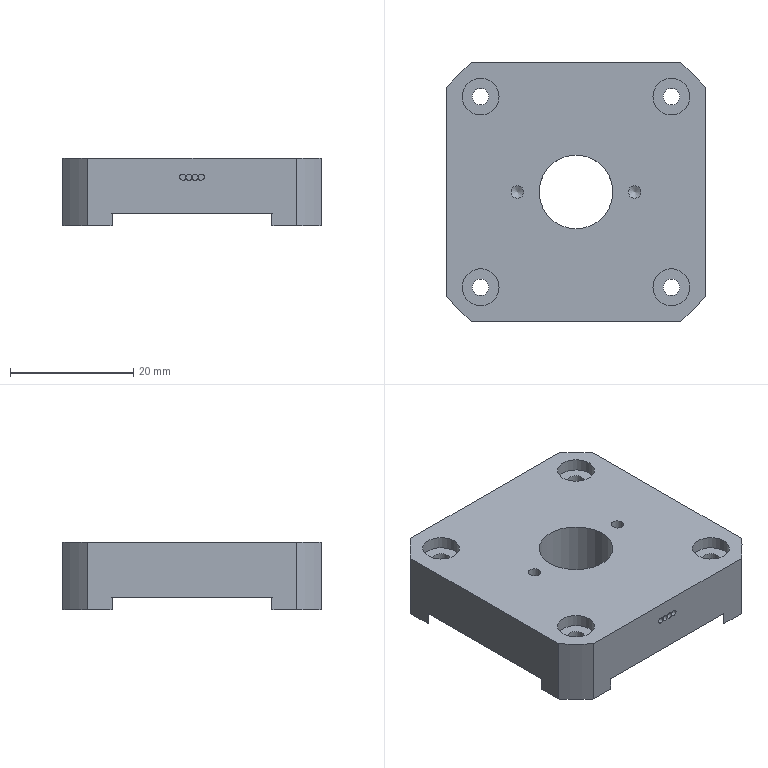Part | NX | 1 solid | 43 faces | box 42 x 42 x 11 mm | volume 14366 mm3 | plane 22 | cylinder 19 | cone 2 | commonest cylinder face diameters 1 x4 2.7 x4 6 x4 54 x4 2.013 x2 12 x1
STEP:
#1=CARTESIAN_POINT('',(-1.,-21.,7.9));
#2=VERTEX_POINT('',#1);
#3=CARTESIAN_POINT('',(-1.5,-21.,7.9));
#4=DIRECTION('',(0.,-1.,0.));
#5=DIRECTION('',(0.,0.,-1.));
#6=AXIS2_PLACEMENT_3D('',#3,#4,#5);
#7=CIRCLE('',#6,0.5);
#8=EDGE_CURVE('',#2,#2,#7,.T.);
#9=ORIENTED_EDGE('',*,*,#8,.T.);
#10=EDGE_LOOP('',(#9));
#11=FACE_BOUND('',#10,.T.);
#12=CARTESIAN_POINT('',(-1.5,-18.,7.4));
#13=VERTEX_POINT('',#12);
#14=CARTESIAN_POINT('',(-1.5,-18.,7.9));
#15=DIRECTION('',(0.,-1.,0.));
#16=DIRECTION('',(0.,0.,-1.));
#17=AXIS2_PLACEMENT_3D('',#14,#15,#16);
#18=CIRCLE('',#17,0.5);
#19=EDGE_CURVE('',#13,#13,#18,.T.);
#20=ORIENTED_EDGE('',*,*,#19,.F.);
#21=EDGE_LOOP('',(#20));
#22=FACE_BOUND('',#21,.T.);
#23=CARTESIAN_POINT('',(-1.5,-19.5,7.9));
#24=DIRECTION('',(0.,-1.,0.));
#25=DIRECTION('',(0.,0.,-1.));
#26=AXIS2_PLACEMENT_3D('',#23,#24,#25);
#27=CYLINDRICAL_SURFACE('',#26,0.5);
#28=ADVANCED_FACE('',(#11,#22),#27,.F.);
#29=ORIENTED_EDGE('',*,*,#19,.T.);
#30=EDGE_LOOP('',(#29));
#31=FACE_BOUND('',#30,.T.);
#32=CARTESIAN_POINT('',(-1.5,-18.,8.4));
#33=DIRECTION('',(0.,1.,0.));
#34=DIRECTION('',(0.,0.,1.));
#35=AXIS2_PLACEMENT_3D('',#32,#33,#34);
#36=PLANE('',#35);
#37=ADVANCED_FACE('',(#31),#36,.F.);
#38=CARTESIAN_POINT('',(-0.5,-18.,7.4));
#39=VERTEX_POINT('',#38);
#40=CARTESIAN_POINT('',(-0.5,-18.,7.9));
#41=DIRECTION('',(0.,-1.,0.));
#42=DIRECTION('',(0.,0.,-1.));
#43=AXIS2_PLACEMENT_3D('',#40,#41,#42);
#44=CIRCLE('',#43,0.5);
#45=EDGE_CURVE('',#39,#39,#44,.T.);
#46=ORIENTED_EDGE('',*,*,#45,.T.);
#47=EDGE_LOOP('',(#46));
#48=FACE_BOUND('',#47,.T.);
#49=CARTESIAN_POINT('',(-0.5,-18.,8.4));
#50=DIRECTION('',(0.,1.,0.));
#51=DIRECTION('',(0.,0.,1.));
#52=AXIS2_PLACEMENT_3D('',#49,#50,#51);
#53=PLANE('',#52);
#54=ADVANCED_FACE('',(#48),#53,.F.);
#55=CARTESIAN_POINT('',(1.5,-18.,7.4));
#56=VERTEX_POINT('',#55);
#57=CARTESIAN_POINT('',(1.5,-18.,7.9));
#58=DIRECTION('',(0.,-1.,0.));
#59=DIRECTION('',(0.,0.,-1.));
#60=AXIS2_PLACEMENT_3D('',#57,#58,#59);
#61=CIRCLE('',#60,0.5);
#62=EDGE_CURVE('',#56,#56,#61,.T.);
#63=ORIENTED_EDGE('',*,*,#62,.T.);
#64=EDGE_LOOP('',(#63));
#65=FACE_BOUND('',#64,.T.);
#66=CARTESIAN_POINT('',(1.5,-18.,8.4));
#67=DIRECTION('',(0.,1.,0.));
#68=DIRECTION('',(0.,0.,1.));
#69=AXIS2_PLACEMENT_3D('',#66,#67,#68);
#70=PLANE('',#69);
#71=ADVANCED_FACE('',(#65),#70,.F.);
#72=CARTESIAN_POINT('',(-9.525,0.,7.395));
#73=VERTEX_POINT('',#72);
#74=VERTEX_LOOP('',#73);
#75=FACE_BOUND('',#74,.T.);
#76=CARTESIAN_POINT('',(-8.518,0.,8.));
#77=VERTEX_POINT('',#76);
#78=CARTESIAN_POINT('',(-9.525,0.,8.));
#79=DIRECTION('',(0.,0.,1.));
#80=DIRECTION('',(1.,0.,0.));
#81=AXIS2_PLACEMENT_3D('',#78,#79,#80);
#82=CIRCLE('',#81,1.006);
#83=EDGE_CURVE('',#77,#77,#82,.T.);
#84=ORIENTED_EDGE('',*,*,#83,.T.);
#85=EDGE_LOOP('',(#84));
#86=FACE_BOUND('',#85,.T.);
#87=CARTESIAN_POINT('',(-9.525,0.,8.));
#88=DIRECTION('',(0.,0.,1.));
#89=DIRECTION('',(1.,0.,0.));
#90=AXIS2_PLACEMENT_3D('',#87,#88,#89);
#91=CONICAL_SURFACE('',#90,1.007,1.03);
#92=ADVANCED_FACE('',(#75,#86),#91,.F.);
#93=CARTESIAN_POINT('',(9.525,0.,7.395));
#94=VERTEX_POINT('',#93);
#95=VERTEX_LOOP('',#94);
#96=FACE_BOUND('',#95,.T.);
#97=CARTESIAN_POINT('',(10.531,0.,8.));
#98=VERTEX_POINT('',#97);
#99=CARTESIAN_POINT('',(9.525,0.,8.));
#100=DIRECTION('',(0.,0.,1.));
#101=DIRECTION('',(1.,0.,0.));
#102=AXIS2_PLACEMENT_3D('',#99,#100,#101);
#103=CIRCLE('',#102,1.006);
#104=EDGE_CURVE('',#98,#98,#103,.T.);
#105=ORIENTED_EDGE('',*,*,#104,.T.);
#106=EDGE_LOOP('',(#105));
#107=FACE_BOUND('',#106,.T.);
#108=CARTESIAN_POINT('',(9.525,0.,8.));
#109=DIRECTION('',(0.,0.,1.));
#110=DIRECTION('',(1.,0.,0.));
#111=AXIS2_PLACEMENT_3D('',#108,#109,#110);
#112=CONICAL_SURFACE('',#111,1.006,1.03);
#113=ADVANCED_FACE('',(#96,#107),#112,.F.);
#114=CARTESIAN_POINT('',(-14.15,15.5,9.));
#115=VERTEX_POINT('',#114);
#116=CARTESIAN_POINT('',(-15.5,15.5,9.));
#117=DIRECTION('',(0.,0.,1.));
#118=DIRECTION('',(1.,0.,0.));
#119=AXIS2_PLACEMENT_3D('',#116,#117,#118);
#120=CIRCLE('',#119,1.35);
#121=EDGE_CURVE('',#115,#115,#120,.T.);
#122=ORIENTED_EDGE('',*,*,#121,.F.);
#123=EDGE_LOOP('',(#122));
#124=FACE_BOUND('',#123,.T.);
#125=CARTESIAN_POINT('',(-12.5,15.5,9.));
#126=VERTEX_POINT('',#125);
#127=CARTESIAN_POINT('',(-15.5,15.5,9.));
#128=DIRECTION('',(0.,0.,1.));
#129=DIRECTION('',(1.,0.,0.));
#130=AXIS2_PLACEMENT_3D('',#127,#128,#129);
#131=CIRCLE('',#130,3.);
#132=EDGE_CURVE('',#126,#126,#131,.T.);
#133=ORIENTED_EDGE('',*,*,#132,.T.);
#134=EDGE_LOOP('',(#133));
#135=FACE_BOUND('',#134,.T.);
#136=CARTESIAN_POINT('',(-15.5,18.5,9.));
#137=DIRECTION('',(0.,0.,-1.));
#138=DIRECTION('',(-1.,0.,0.));
#139=AXIS2_PLACEMENT_3D('',#136,#137,#138);
#140=PLANE('',#139);
#141=ADVANCED_FACE('',(#124,#135),#140,.F.);
#142=CARTESIAN_POINT('',(16.85,15.5,9.));
#143=VERTEX_POINT('',#142);
#144=CARTESIAN_POINT('',(15.5,15.5,9.));
#145=DIRECTION('',(0.,0.,1.));
#146=DIRECTION('',(1.,0.,0.));
#147=AXIS2_PLACEMENT_3D('',#144,#145,#146);
#148=CIRCLE('',#147,1.35);
#149=EDGE_CURVE('',#143,#143,#148,.T.);
#150=ORIENTED_EDGE('',*,*,#149,.F.);
#151=EDGE_LOOP('',(#150));
#152=FACE_BOUND('',#151,.T.);
#153=CARTESIAN_POINT('',(18.5,15.5,9.));
#154=VERTEX_POINT('',#153);
#155=CARTESIAN_POINT('',(15.5,15.5,9.));
#156=DIRECTION('',(0.,0.,1.));
#157=DIRECTION('',(1.,0.,0.));
#158=AXIS2_PLACEMENT_3D('',#155,#156,#157);
#159=CIRCLE('',#158,3.);
#160=EDGE_CURVE('',#154,#154,#159,.T.);
#161=ORIENTED_EDGE('',*,*,#160,.T.);
#162=EDGE_LOOP('',(#161));
#163=FACE_BOUND('',#162,.T.);
#164=CARTESIAN_POINT('',(15.5,18.5,9.));
#165=DIRECTION('',(0.,0.,-1.));
#166=DIRECTION('',(-1.,0.,0.));
#167=AXIS2_PLACEMENT_3D('',#164,#165,#166);
#168=PLANE('',#167);
#169=ADVANCED_FACE('',(#152,#163),#168,.F.);
#170=CARTESIAN_POINT('',(-14.15,-15.5,9.));
#171=VERTEX_POINT('',#170);
#172=CARTESIAN_POINT('',(-15.5,-15.5,9.));
#173=DIRECTION('',(0.,0.,1.));
#174=DIRECTION('',(1.,0.,0.));
#175=AXIS2_PLACEMENT_3D('',#172,#173,#174);
#176=CIRCLE('',#175,1.35);
#177=EDGE_CURVE('',#171,#171,#176,.T.);
#178=ORIENTED_EDGE('',*,*,#177,.F.);
#179=EDGE_LOOP('',(#178));
#180=FACE_BOUND('',#179,.T.);
#181=CARTESIAN_POINT('',(-12.5,-15.5,9.));
#182=VERTEX_POINT('',#181);
#183=CARTESIAN_POINT('',(-15.5,-15.5,9.));
#184=DIRECTION('',(0.,0.,1.));
#185=DIRECTION('',(1.,0.,0.));
#186=AXIS2_PLACEMENT_3D('',#183,#184,#185);
#187=CIRCLE('',#186,3.);
#188=EDGE_CURVE('',#182,#182,#187,.T.);
#189=ORIENTED_EDGE('',*,*,#188,.T.);
#190=EDGE_LOOP('',(#189));
#191=FACE_BOUND('',#190,.T.);
#192=CARTESIAN_POINT('',(-15.5,-12.5,9.));
#193=DIRECTION('',(0.,0.,-1.));
#194=DIRECTION('',(-1.,0.,0.));
#195=AXIS2_PLACEMENT_3D('',#192,#193,#194);
#196=PLANE('',#195);
#197=ADVANCED_FACE('',(#180,#191),#196,.F.);
#198=CARTESIAN_POINT('',(16.85,-15.5,9.));
#199=VERTEX_POINT('',#198);
#200=CARTESIAN_POINT('',(15.5,-15.5,9.));
#201=DIRECTION('',(0.,0.,1.));
#202=DIRECTION('',(1.,0.,0.));
#203=AXIS2_PLACEMENT_3D('',#200,#201,#202);
#204=CIRCLE('',#203,1.35);
#205=EDGE_CURVE('',#199,#199,#204,.T.);
#206=ORIENTED_EDGE('',*,*,#205,.F.);
#207=EDGE_LOOP('',(#206));
#208=FACE_BOUND('',#207,.T.);
#209=CARTESIAN_POINT('',(18.5,-15.5,9.));
#210=VERTEX_POINT('',#209);
#211=CARTESIAN_POINT('',(15.5,-15.5,9.));
#212=DIRECTION('',(0.,0.,1.));
#213=DIRECTION('',(1.,0.,0.));
#214=AXIS2_PLACEMENT_3D('',#211,#212,#213);
#215=CIRCLE('',#214,3.);
#216=EDGE_CURVE('',#210,#210,#215,.T.);
#217=ORIENTED_EDGE('',*,*,#216,.T.);
#218=EDGE_LOOP('',(#217));
#219=FACE_BOUND('',#218,.T.);
#220=CARTESIAN_POINT('',(15.5,-12.5,9.));
#221=DIRECTION('',(0.,0.,-1.));
#222=DIRECTION('',(-1.,0.,0.));
#223=AXIS2_PLACEMENT_3D('',#220,#221,#222);
#224=PLANE('',#223);
#225=ADVANCED_FACE('',(#208,#219),#224,.F.);
#226=CARTESIAN_POINT('',(16.971,21.,0.));
#227=VERTEX_POINT('',#226);
#228=CARTESIAN_POINT('',(13.,21.,0.));
#229=VERTEX_POINT('',#228);
#230=CARTESIAN_POINT('',(-16.971,21.,0.));
#231=DIRECTION('',(1.,0.,0.));
#232=VECTOR('',#231,1000.);
#233=LINE('',#230,#232);
#234=EDGE_CURVE('',#227,#229,#233,.F.);
#235=ORIENTED_EDGE('',*,*,#234,.F.);
#236=CARTESIAN_POINT('',(21.,16.971,0.));
#237=VERTEX_POINT('',#236);
#238=CARTESIAN_POINT('',(0.,0.,0.));
#239=DIRECTION('',(0.,0.,1.));
#240=DIRECTION('',(1.,0.,0.));
#241=AXIS2_PLACEMENT_3D('',#238,#239,#240);
#242=CIRCLE('',#241,27.);
#243=EDGE_CURVE('',#237,#227,#242,.T.);
#244=ORIENTED_EDGE('',*,*,#243,.F.);
#245=CARTESIAN_POINT('',(21.,13.,0.));
#246=VERTEX_POINT('',#245);
#247=CARTESIAN_POINT('',(21.,16.971,0.));
#248=DIRECTION('',(0.,1.,0.));
#249=VECTOR('',#248,1000.);
#250=LINE('',#247,#249);
#251=EDGE_CURVE('',#246,#237,#250,.T.);
#252=ORIENTED_EDGE('',*,*,#251,.F.);
#253=CARTESIAN_POINT('',(13.,21.,0.));
#254=DIRECTION('',(0.7071,-0.7071,0.));
#255=VECTOR('',#254,1000.);
#256=LINE('',#253,#255);
#257=EDGE_CURVE('',#229,#246,#256,.T.);
#258=ORIENTED_EDGE('',*,*,#257,.F.);
#259=EDGE_LOOP('',(#235,#244,#252,#258));
#260=FACE_BOUND('',#259,.T.);
#261=CARTESIAN_POINT('',(0.,0.,0.));
#262=DIRECTION('',(0.,0.,1.));
#263=DIRECTION('',(1.,0.,0.));
#264=AXIS2_PLACEMENT_3D('',#261,#262,#263);
#265=PLANE('',#264);
#266=ADVANCED_FACE('',(#260),#265,.F.);
#267=CARTESIAN_POINT('',(-21.,16.971,0.));
#268=VERTEX_POINT('',#267);
#269=CARTESIAN_POINT('',(-21.,13.,0.));
#270=VERTEX_POINT('',#269);
#271=CARTESIAN_POINT('',(-21.,-16.971,0.));
#272=DIRECTION('',(0.,1.,0.));
#273=VECTOR('',#272,1000.);
#274=LINE('',#271,#273);
#275=EDGE_CURVE('',#268,#270,#274,.F.);
#276=ORIENTED_EDGE('',*,*,#275,.F.);
#277=CARTESIAN_POINT('',(-16.971,21.,0.));
#278=VERTEX_POINT('',#277);
#279=CARTESIAN_POINT('',(0.,0.,0.));
#280=DIRECTION('',(0.,0.,1.));
#281=DIRECTION('',(1.,0.,0.));
#282=AXIS2_PLACEMENT_3D('',#279,#280,#281);
#283=CIRCLE('',#282,27.);
#284=EDGE_CURVE('',#278,#268,#283,.T.);
#285=ORIENTED_EDGE('',*,*,#284,.F.);
#286=CARTESIAN_POINT('',(-13.,21.,0.));
#287=VERTEX_POINT('',#286);
#288=CARTESIAN_POINT('',(-16.971,21.,0.));
#289=DIRECTION('',(1.,0.,0.));
#290=VECTOR('',#289,1000.);
#291=LINE('',#288,#290);
#292=EDGE_CURVE('',#287,#278,#291,.F.);
#293=ORIENTED_EDGE('',*,*,#292,.F.);
#294=CARTESIAN_POINT('',(-21.,13.,0.));
#295=DIRECTION('',(-0.7071,-0.7071,0.));
#296=VECTOR('',#295,1000.);
#297=LINE('',#294,#296);
#298=EDGE_CURVE('',#287,#270,#297,.T.);
#299=ORIENTED_EDGE('',*,*,#298,.T.);
#300=EDGE_LOOP('',(#276,#285,#293,#299));
#301=FACE_BOUND('',#300,.T.);
#302=CARTESIAN_POINT('',(0.,0.,0.));
#303=DIRECTION('',(0.,0.,1.));
#304=DIRECTION('',(1.,0.,0.));
#305=AXIS2_PLACEMENT_3D('',#302,#303,#304);
#306=PLANE('',#305);
#307=ADVANCED_FACE('',(#301),#306,.F.);
#308=ORIENTED_EDGE('',*,*,#284,.T.);
#309=CARTESIAN_POINT('',(-21.,16.971,11.));
#310=VERTEX_POINT('',#309);
#311=CARTESIAN_POINT('',(-21.,16.971,0.));
#312=DIRECTION('',(0.,0.,1.));
#313=VECTOR('',#312,1000.);
#314=LINE('',#311,#313);
#315=EDGE_CURVE('',#310,#268,#314,.F.);
#316=ORIENTED_EDGE('',*,*,#315,.F.);
#317=CARTESIAN_POINT('',(-16.971,21.,11.));
#318=VERTEX_POINT('',#317);
#319=CARTESIAN_POINT('',(0.,0.,11.));
#320=DIRECTION('',(0.,0.,1.));
#321=DIRECTION('',(1.,0.,0.));
#322=AXIS2_PLACEMENT_3D('',#319,#320,#321);
#323=CIRCLE('',#322,27.);
#324=EDGE_CURVE('',#318,#310,#323,.T.);
#325=ORIENTED_EDGE('',*,*,#324,.F.);
#326=CARTESIAN_POINT('',(-16.971,21.,0.));
#327=DIRECTION('',(0.,0.,1.));
#328=VECTOR('',#327,1000.);
#329=LINE('',#326,#328);
#330=EDGE_CURVE('',#318,#278,#329,.F.);
#331=ORIENTED_EDGE('',*,*,#330,.T.);
#332=EDGE_LOOP('',(#308,#316,#325,#331));
#333=FACE_BOUND('',#332,.T.);
#334=CARTESIAN_POINT('',(0.,0.,0.));
#335=DIRECTION('',(0.,0.,1.));
#336=DIRECTION('',(1.,0.,0.));
#337=AXIS2_PLACEMENT_3D('',#334,#335,#336);
#338=CYLINDRICAL_SURFACE('',#337,27.);
#339=ADVANCED_FACE('',(#333),#338,.T.);
#340=ORIENTED_EDGE('',*,*,#243,.T.);
#341=CARTESIAN_POINT('',(16.971,21.,11.));
#342=VERTEX_POINT('',#341);
#343=CARTESIAN_POINT('',(16.971,21.,0.));
#344=DIRECTION('',(0.,0.,1.));
#345=VECTOR('',#344,1000.);
#346=LINE('',#343,#345);
#347=EDGE_CURVE('',#227,#342,#346,.T.);
#348=ORIENTED_EDGE('',*,*,#347,.T.);
#349=CARTESIAN_POINT('',(21.,16.971,11.));
#350=VERTEX_POINT('',#349);
#351=CARTESIAN_POINT('',(0.,0.,11.));
#352=DIRECTION('',(0.,0.,1.));
#353=DIRECTION('',(1.,0.,0.));
#354=AXIS2_PLACEMENT_3D('',#351,#352,#353);
#355=CIRCLE('',#354,27.);
#356=EDGE_CURVE('',#350,#342,#355,.T.);
#357=ORIENTED_EDGE('',*,*,#356,.F.);
#358=CARTESIAN_POINT('',(21.,16.971,0.));
#359=DIRECTION('',(0.,0.,1.));
#360=VECTOR('',#359,1000.);
#361=LINE('',#358,#360);
#362=EDGE_CURVE('',#350,#237,#361,.F.);
#363=ORIENTED_EDGE('',*,*,#362,.T.);
#364=EDGE_LOOP('',(#340,#348,#357,#363));
#365=FACE_BOUND('',#364,.T.);
#366=CARTESIAN_POINT('',(0.,0.,0.));
#367=DIRECTION('',(0.,0.,1.));
#368=DIRECTION('',(1.,0.,0.));
#369=AXIS2_PLACEMENT_3D('',#366,#367,#368);
#370=CYLINDRICAL_SURFACE('',#369,27.);
#371=ADVANCED_FACE('',(#365),#370,.T.);
#372=ORIENTED_EDGE('',*,*,#83,.F.);
#373=EDGE_LOOP('',(#372));
#374=FACE_BOUND('',#373,.T.);
#375=CARTESIAN_POINT('',(-8.518,0.,11.));
#376=VERTEX_POINT('',#375);
#377=CARTESIAN_POINT('',(-9.525,0.,11.));
#378=DIRECTION('',(0.,0.,1.));
#379=DIRECTION('',(1.,0.,0.));
#380=AXIS2_PLACEMENT_3D('',#377,#378,#379);
#381=CIRCLE('',#380,1.006);
#382=EDGE_CURVE('',#376,#376,#381,.F.);
#383=ORIENTED_EDGE('',*,*,#382,.F.);
#384=EDGE_LOOP('',(#383));
#385=FACE_BOUND('',#384,.T.);
#386=CARTESIAN_POINT('',(-9.525,0.,9.5));
#387=DIRECTION('',(0.,0.,1.));
#388=DIRECTION('',(1.,0.,0.));
#389=AXIS2_PLACEMENT_3D('',#386,#387,#388);
#390=CYLINDRICAL_SURFACE('',#389,1.006);
#391=ADVANCED_FACE('',(#374,#385),#390,.F.);
#392=ORIENTED_EDGE('',*,*,#104,.F.);
#393=EDGE_LOOP('',(#392));
#394=FACE_BOUND('',#393,.T.);
#395=CARTESIAN_POINT('',(10.531,0.,11.));
#396=VERTEX_POINT('',#395);
#397=CARTESIAN_POINT('',(9.525,0.,11.));
#398=DIRECTION('',(0.,0.,1.));
#399=DIRECTION('',(1.,0.,0.));
#400=AXIS2_PLACEMENT_3D('',#397,#398,#399);
#401=CIRCLE('',#400,1.006);
#402=EDGE_CURVE('',#396,#396,#401,.F.);
#403=ORIENTED_EDGE('',*,*,#402,.F.);
#404=EDGE_LOOP('',(#403));
#405=FACE_BOUND('',#404,.T.);
#406=CARTESIAN_POINT('',(9.525,0.,9.5));
#407=DIRECTION('',(0.,0.,1.));
#408=DIRECTION('',(1.,0.,0.));
#409=AXIS2_PLACEMENT_3D('',#406,#407,#408);
#410=CYLINDRICAL_SURFACE('',#409,1.006);
#411=ADVANCED_FACE('',(#394,#405),#410,.F.);
#412=ORIENTED_EDGE('',*,*,#132,.F.);
#413=EDGE_LOOP('',(#412));
#414=FACE_BOUND('',#413,.T.);
#415=CARTESIAN_POINT('',(-12.5,15.5,11.));
#416=VERTEX_POINT('',#415);
#417=CARTESIAN_POINT('',(-15.5,15.5,11.));
#418=DIRECTION('',(0.,0.,1.));
#419=DIRECTION('',(1.,0.,0.));
#420=AXIS2_PLACEMENT_3D('',#417,#418,#419);
#421=CIRCLE('',#420,3.);
#422=EDGE_CURVE('',#416,#416,#421,.F.);
#423=ORIENTED_EDGE('',*,*,#422,.F.);
#424=EDGE_LOOP('',(#423));
#425=FACE_BOUND('',#424,.T.);
#426=CARTESIAN_POINT('',(-15.5,15.5,10.));
#427=DIRECTION('',(0.,0.,1.));
#428=DIRECTION('',(1.,0.,0.));
#429=AXIS2_PLACEMENT_3D('',#426,#427,#428);
#430=CYLINDRICAL_SURFACE('',#429,3.);
#431=ADVANCED_FACE('',(#414,#425),#430,.F.);
#432=ORIENTED_EDGE('',*,*,#160,.F.);
#433=EDGE_LOOP('',(#432));
#434=FACE_BOUND('',#433,.T.);
#435=CARTESIAN_POINT('',(18.5,15.5,11.));
#436=VERTEX_POINT('',#435);
#437=CARTESIAN_POINT('',(15.5,15.5,11.));
#438=DIRECTION('',(0.,0.,1.));
#439=DIRECTION('',(1.,0.,0.));
#440=AXIS2_PLACEMENT_3D('',#437,#438,#439);
#441=CIRCLE('',#440,3.);
#442=EDGE_CURVE('',#436,#436,#441,.F.);
#443=ORIENTED_EDGE('',*,*,#442,.F.);
#444=EDGE_LOOP('',(#443));
#445=FACE_BOUND('',#444,.T.);
#446=CARTESIAN_POINT('',(15.5,15.5,10.));
#447=DIRECTION('',(0.,0.,1.));
#448=DIRECTION('',(1.,0.,0.));
#449=AXIS2_PLACEMENT_3D('',#446,#447,#448);
#450=CYLINDRICAL_SURFACE('',#449,3.);
#451=ADVANCED_FACE('',(#434,#445),#450,.F.);
#452=ORIENTED_EDGE('',*,*,#188,.F.);
#453=EDGE_LOOP('',(#452));
#454=FACE_BOUND('',#453,.T.);
#455=CARTESIAN_POINT('',(-12.5,-15.5,11.));
#456=VERTEX_POINT('',#455);
#457=CARTESIAN_POINT('',(-15.5,-15.5,11.));
#458=DIRECTION('',(0.,0.,1.));
#459=DIRECTION('',(1.,0.,0.));
#460=AXIS2_PLACEMENT_3D('',#457,#458,#459);
#461=CIRCLE('',#460,3.);
#462=EDGE_CURVE('',#456,#456,#461,.F.);
#463=ORIENTED_EDGE('',*,*,#462,.F.);
#464=EDGE_LOOP('',(#463));
#465=FACE_BOUND('',#464,.T.);
#466=CARTESIAN_POINT('',(-15.5,-15.5,10.));
#467=DIRECTION('',(0.,0.,1.));
#468=DIRECTION('',(1.,0.,0.));
#469=AXIS2_PLACEMENT_3D('',#466,#467,#468);
#470=CYLINDRICAL_SURFACE('',#469,3.);
#471=ADVANCED_FACE('',(#454,#465),#470,.F.);
#472=ORIENTED_EDGE('',*,*,#216,.F.);
#473=EDGE_LOOP('',(#472));
#474=FACE_BOUND('',#473,.T.);
#475=CARTESIAN_POINT('',(18.5,-15.5,11.));
#476=VERTEX_POINT('',#475);
#477=CARTESIAN_POINT('',(15.5,-15.5,11.));
#478=DIRECTION('',(0.,0.,1.));
#479=DIRECTION('',(1.,0.,0.));
#480=AXIS2_PLACEMENT_3D('',#477,#478,#479);
#481=CIRCLE('',#480,3.);
#482=EDGE_CURVE('',#476,#476,#481,.F.);
#483=ORIENTED_EDGE('',*,*,#482,.F.);
#484=EDGE_LOOP('',(#483));
#485=FACE_BOUND('',#484,.T.);
#486=CARTESIAN_POINT('',(15.5,-15.5,10.));
#487=DIRECTION('',(0.,0.,1.));
#488=DIRECTION('',(1.,0.,0.));
#489=AXIS2_PLACEMENT_3D('',#486,#487,#488);
#490=CYLINDRICAL_SURFACE('',#489,3.);
#491=ADVANCED_FACE('',(#474,#485),#490,.F.);
#492=CARTESIAN_POINT('',(13.,21.,2.));
#493=VERTEX_POINT('',#492);
#494=CARTESIAN_POINT('',(13.,21.,0.));
#495=DIRECTION('',(0.,0.,1.));
#496=VECTOR('',#495,1000.);
#497=LINE('',#494,#496);
#498=EDGE_CURVE('',#229,#493,#497,.T.);
#499=ORIENTED_EDGE('',*,*,#498,.F.);
#500=ORIENTED_EDGE('',*,*,#257,.T.);
#501=CARTESIAN_POINT('',(21.,13.,2.));
#502=VERTEX_POINT('',#501);
#503=CARTESIAN_POINT('',(21.,13.,0.));
#504=DIRECTION('',(0.,0.,-1.));
#505=VECTOR('',#504,1000.);
#506=LINE('',#503,#505);
#507=EDGE_CURVE('',#502,#246,#506,.T.);
#508=ORIENTED_EDGE('',*,*,#507,.F.);
#509=CARTESIAN_POINT('',(21.,13.,2.));
#510=DIRECTION('',(-0.7071,0.7071,0.));
#511=VECTOR('',#510,1000.);
#512=LINE('',#509,#511);
#513=EDGE_CURVE('',#502,#493,#512,.T.);
#514=ORIENTED_EDGE('',*,*,#513,.T.);
#515=EDGE_LOOP('',(#499,#500,#508,#514));
#516=FACE_BOUND('',#515,.T.);
#517=CARTESIAN_POINT('',(13.,21.,0.));
#518=DIRECTION('',(0.7071,0.7071,0.));
#519=DIRECTION('',(-0.7071,0.7071,0.));
#520=AXIS2_PLACEMENT_3D('',#517,#518,#519);
#521=PLANE('',#520);
#522=ADVANCED_FACE('',(#516),#521,.F.);
#523=ORIENTED_EDGE('',*,*,#347,.F.);
#524=ORIENTED_EDGE('',*,*,#234,.T.);
#525=ORIENTED_EDGE('',*,*,#498,.T.);
#526=CARTESIAN_POINT('',(-13.,21.,2.));
#527=VERTEX_POINT('',#526);
#528=CARTESIAN_POINT('',(-16.971,21.,2.));
#529=DIRECTION('',(1.,0.,0.));
#530=VECTOR('',#529,1000.);
#531=LINE('',#528,#530);
#532=EDGE_CURVE('',#493,#527,#531,.F.);
#533=ORIENTED_EDGE('',*,*,#532,.T.);
#534=CARTESIAN_POINT('',(-13.,21.,0.));
#535=DIRECTION('',(0.,0.,1.));
#536=VECTOR('',#535,1000.);
#537=LINE('',#534,#536);
#538=EDGE_CURVE('',#527,#287,#537,.F.);
#539=ORIENTED_EDGE('',*,*,#538,.T.);
#540=ORIENTED_EDGE('',*,*,#292,.T.);
#541=ORIENTED_EDGE('',*,*,#330,.F.);
#542=CARTESIAN_POINT('',(0.,21.,11.));
#543=DIRECTION('',(1.,0.,0.));
#544=VECTOR('',#543,1000.);
#545=LINE('',#542,#544);
#546=EDGE_CURVE('',#342,#318,#545,.F.);
#547=ORIENTED_EDGE('',*,*,#546,.F.);
#548=EDGE_LOOP('',(#523,#524,#525,#533,#539,#540,#541,#547));
#549=FACE_BOUND('',#548,.T.);
#550=CARTESIAN_POINT('',(-16.971,21.,0.));
#551=DIRECTION('',(0.,1.,0.));
#552=DIRECTION('',(0.,0.,1.));
#553=AXIS2_PLACEMENT_3D('',#550,#551,#552);
#554=PLANE('',#553);
#555=ADVANCED_FACE('',(#549),#554,.T.);
#556=CARTESIAN_POINT('',(-21.,13.,2.));
#557=VERTEX_POINT('',#556);
#558=CARTESIAN_POINT('',(-21.,13.,0.));
#559=DIRECTION('',(0.,0.,1.));
#560=VECTOR('',#559,1000.);
#561=LINE('',#558,#560);
#562=EDGE_CURVE('',#270,#557,#561,.T.);
#563=ORIENTED_EDGE('',*,*,#562,.F.);
#564=ORIENTED_EDGE('',*,*,#298,.F.);
#565=ORIENTED_EDGE('',*,*,#538,.F.);
#566=CARTESIAN_POINT('',(-13.,21.,2.));
#567=DIRECTION('',(-0.7071,-0.7071,0.));
#568=VECTOR('',#567,1000.);
#569=LINE('',#566,#568);
#570=EDGE_CURVE('',#527,#557,#569,.T.);
#571=ORIENTED_EDGE('',*,*,#570,.T.);
#572=EDGE_LOOP('',(#563,#564,#565,#571));
#573=FACE_BOUND('',#572,.T.);
#574=CARTESIAN_POINT('',(-21.,13.,0.));
#575=DIRECTION('',(-0.7071,0.7071,0.));
#576=DIRECTION('',(-0.7071,-0.7071,0.));
#577=AXIS2_PLACEMENT_3D('',#574,#575,#576);
#578=PLANE('',#577);
#579=ADVANCED_FACE('',(#573),#578,.F.);
#580=CARTESIAN_POINT('',(-6.,0.,11.));
#581=VERTEX_POINT('',#580);
#582=CARTESIAN_POINT('',(0.,0.,11.));
#583=DIRECTION('',(0.,0.,-1.));
#584=DIRECTION('',(-1.,0.,0.));
#585=AXIS2_PLACEMENT_3D('',#582,#583,#584);
#586=CIRCLE('',#585,6.);
#587=EDGE_CURVE('',#581,#581,#586,.T.);
#588=ORIENTED_EDGE('',*,*,#587,.F.);
#589=EDGE_LOOP('',(#588));
#590=FACE_BOUND('',#589,.T.);
#591=CARTESIAN_POINT('',(-6.,0.,2.));
#592=VERTEX_POINT('',#591);
#593=CARTESIAN_POINT('',(0.,0.,2.));
#594=DIRECTION('',(0.,0.,-1.));
#595=DIRECTION('',(-1.,0.,0.));
#596=AXIS2_PLACEMENT_3D('',#593,#594,#595);
#597=CIRCLE('',#596,6.);
#598=EDGE_CURVE('',#592,#592,#597,.F.);
#599=ORIENTED_EDGE('',*,*,#598,.F.);
#600=EDGE_LOOP('',(#599));
#601=FACE_BOUND('',#600,.T.);
#602=CARTESIAN_POINT('',(0.,0.,11.));
#603=DIRECTION('',(0.,0.,-1.));
#604=DIRECTION('',(-1.,0.,0.));
#605=AXIS2_PLACEMENT_3D('',#602,#603,#604);
#606=CYLINDRICAL_SURFACE('',#605,6.);
#607=ADVANCED_FACE('',(#590,#601),#606,.F.);
#608=ORIENTED_EDGE('',*,*,#121,.T.);
#609=EDGE_LOOP('',(#608));
#610=FACE_BOUND('',#609,.T.);
#611=CARTESIAN_POINT('',(-14.15,15.5,2.));
#612=VERTEX_POINT('',#611);
#613=CARTESIAN_POINT('',(-15.5,15.5,2.));
#614=DIRECTION('',(0.,0.,1.));
#615=DIRECTION('',(1.,0.,0.));
#616=AXIS2_PLACEMENT_3D('',#613,#614,#615);
#617=CIRCLE('',#616,1.35);
#618=EDGE_CURVE('',#612,#612,#617,.F.);
#619=ORIENTED_EDGE('',*,*,#618,.T.);
#620=EDGE_LOOP('',(#619));
#621=FACE_BOUND('',#620,.T.);
#622=CARTESIAN_POINT('',(-15.5,15.5,5.5));
#623=DIRECTION('',(0.,0.,1.));
#624=DIRECTION('',(1.,0.,0.));
#625=AXIS2_PLACEMENT_3D('',#622,#623,#624);
#626=CYLINDRICAL_SURFACE('',#625,1.35);
#627=ADVANCED_FACE('',(#610,#621),#626,.F.);
#628=ORIENTED_EDGE('',*,*,#149,.T.);
#629=EDGE_LOOP('',(#628));
#630=FACE_BOUND('',#629,.T.);
#631=CARTESIAN_POINT('',(16.85,15.5,2.));
#632=VERTEX_POINT('',#631);
#633=CARTESIAN_POINT('',(15.5,15.5,2.));
#634=DIRECTION('',(0.,0.,1.));
#635=DIRECTION('',(1.,0.,0.));
#636=AXIS2_PLACEMENT_3D('',#633,#634,#635);
#637=CIRCLE('',#636,1.35);
#638=EDGE_CURVE('',#632,#632,#637,.F.);
#639=ORIENTED_EDGE('',*,*,#638,.T.);
#640=EDGE_LOOP('',(#639));
#641=FACE_BOUND('',#640,.T.);
#642=CARTESIAN_POINT('',(15.5,15.5,5.5));
#643=DIRECTION('',(0.,0.,1.));
#644=DIRECTION('',(1.,0.,0.));
#645=AXIS2_PLACEMENT_3D('',#642,#643,#644);
#646=CYLINDRICAL_SURFACE('',#645,1.35);
#647=ADVANCED_FACE('',(#630,#641),#646,.F.);
#648=ORIENTED_EDGE('',*,*,#177,.T.);
#649=EDGE_LOOP('',(#648));
#650=FACE_BOUND('',#649,.T.);
#651=CARTESIAN_POINT('',(-14.15,-15.5,2.));
#652=VERTEX_POINT('',#651);
#653=CARTESIAN_POINT('',(-15.5,-15.5,2.));
#654=DIRECTION('',(0.,0.,1.));
#655=DIRECTION('',(1.,0.,0.));
#656=AXIS2_PLACEMENT_3D('',#653,#654,#655);
#657=CIRCLE('',#656,1.35);
#658=EDGE_CURVE('',#652,#652,#657,.F.);
#659=ORIENTED_EDGE('',*,*,#658,.T.);
#660=EDGE_LOOP('',(#659));
#661=FACE_BOUND('',#660,.T.);
#662=CARTESIAN_POINT('',(-15.5,-15.5,5.5));
#663=DIRECTION('',(0.,0.,1.));
#664=DIRECTION('',(1.,0.,0.));
#665=AXIS2_PLACEMENT_3D('',#662,#663,#664);
#666=CYLINDRICAL_SURFACE('',#665,1.35);
#667=ADVANCED_FACE('',(#650,#661),#666,.F.);
#668=ORIENTED_EDGE('',*,*,#205,.T.);
#669=EDGE_LOOP('',(#668));
#670=FACE_BOUND('',#669,.T.);
#671=CARTESIAN_POINT('',(16.85,-15.5,2.));
#672=VERTEX_POINT('',#671);
#673=CARTESIAN_POINT('',(15.5,-15.5,2.));
#674=DIRECTION('',(0.,0.,1.));
#675=DIRECTION('',(1.,0.,0.));
#676=AXIS2_PLACEMENT_3D('',#673,#674,#675);
#677=CIRCLE('',#676,1.35);
#678=EDGE_CURVE('',#672,#672,#677,.F.);
#679=ORIENTED_EDGE('',*,*,#678,.T.);
#680=EDGE_LOOP('',(#679));
#681=FACE_BOUND('',#680,.T.);
#682=CARTESIAN_POINT('',(15.5,-15.5,5.5));
#683=DIRECTION('',(0.,0.,1.));
#684=DIRECTION('',(1.,0.,0.));
#685=AXIS2_PLACEMENT_3D('',#682,#683,#684);
#686=CYLINDRICAL_SURFACE('',#685,1.35);
#687=ADVANCED_FACE('',(#670,#681),#686,.F.);
#688=CARTESIAN_POINT('',(21.,-16.971,11.));
#689=VERTEX_POINT('',#688);
#690=CARTESIAN_POINT('',(21.,-16.971,0.));
#691=VERTEX_POINT('',#690);
#692=CARTESIAN_POINT('',(21.,-16.971,0.));
#693=DIRECTION('',(0.,0.,-1.));
#694=VECTOR('',#693,1000.);
#695=LINE('',#692,#694);
#696=EDGE_CURVE('',#689,#691,#695,.T.);
#697=ORIENTED_EDGE('',*,*,#696,.T.);
#698=CARTESIAN_POINT('',(21.,-13.,0.));
#699=VERTEX_POINT('',#698);
#700=CARTESIAN_POINT('',(21.,16.971,0.));
#701=DIRECTION('',(0.,1.,0.));
#702=VECTOR('',#701,1000.);
#703=LINE('',#700,#702);
#704=EDGE_CURVE('',#691,#699,#703,.T.);
#705=ORIENTED_EDGE('',*,*,#704,.T.);
#706=CARTESIAN_POINT('',(21.,-13.,2.));
#707=VERTEX_POINT('',#706);
#708=CARTESIAN_POINT('',(21.,-13.,0.));
#709=DIRECTION('',(0.,0.,-1.));
#710=VECTOR('',#709,1000.);
#711=LINE('',#708,#710);
#712=EDGE_CURVE('',#699,#707,#711,.F.);
#713=ORIENTED_EDGE('',*,*,#712,.T.);
#714=CARTESIAN_POINT('',(21.,16.971,2.));
#715=DIRECTION('',(0.,1.,0.));
#716=VECTOR('',#715,1000.);
#717=LINE('',#714,#716);
#718=EDGE_CURVE('',#707,#502,#717,.T.);
#719=ORIENTED_EDGE('',*,*,#718,.T.);
#720=ORIENTED_EDGE('',*,*,#507,.T.);
#721=ORIENTED_EDGE('',*,*,#251,.T.);
#722=ORIENTED_EDGE('',*,*,#362,.F.);
#723=CARTESIAN_POINT('',(21.,0.,11.));
#724=DIRECTION('',(0.,1.,0.));
#725=VECTOR('',#724,1000.);
#726=LINE('',#723,#725);
#727=EDGE_CURVE('',#689,#350,#726,.T.);
#728=ORIENTED_EDGE('',*,*,#727,.F.);
#729=EDGE_LOOP('',(#697,#705,#713,#719,#720,#721,#722,#728));
#730=FACE_BOUND('',#729,.T.);
#731=CARTESIAN_POINT('',(21.,16.971,0.));
#732=DIRECTION('',(1.,0.,0.));
#733=DIRECTION('',(0.,0.,-1.));
#734=AXIS2_PLACEMENT_3D('',#731,#732,#733);
#735=PLANE('',#734);
#736=ADVANCED_FACE('',(#730),#735,.T.);
#737=ORIENTED_EDGE('',*,*,#562,.T.);
#738=CARTESIAN_POINT('',(-21.,-13.,2.));
#739=VERTEX_POINT('',#738);
#740=CARTESIAN_POINT('',(-21.,-16.971,2.));
#741=DIRECTION('',(0.,1.,0.));
#742=VECTOR('',#741,1000.);
#743=LINE('',#740,#742);
#744=EDGE_CURVE('',#557,#739,#743,.F.);
#745=ORIENTED_EDGE('',*,*,#744,.T.);
#746=CARTESIAN_POINT('',(-21.,-13.,0.));
#747=VERTEX_POINT('',#746);
#748=CARTESIAN_POINT('',(-21.,-13.,0.));
#749=DIRECTION('',(0.,0.,1.));
#750=VECTOR('',#749,1000.);
#751=LINE('',#748,#750);
#752=EDGE_CURVE('',#739,#747,#751,.F.);
#753=ORIENTED_EDGE('',*,*,#752,.T.);
#754=CARTESIAN_POINT('',(-21.,-16.971,0.));
#755=VERTEX_POINT('',#754);
#756=CARTESIAN_POINT('',(-21.,-16.971,0.));
#757=DIRECTION('',(0.,1.,0.));
#758=VECTOR('',#757,1000.);
#759=LINE('',#756,#758);
#760=EDGE_CURVE('',#747,#755,#759,.F.);
#761=ORIENTED_EDGE('',*,*,#760,.T.);
#762=CARTESIAN_POINT('',(-21.,-16.971,11.));
#763=VERTEX_POINT('',#762);
#764=CARTESIAN_POINT('',(-21.,-16.971,0.));
#765=DIRECTION('',(0.,0.,1.));
#766=VECTOR('',#765,1000.);
#767=LINE('',#764,#766);
#768=EDGE_CURVE('',#763,#755,#767,.F.);
#769=ORIENTED_EDGE('',*,*,#768,.F.);
#770=CARTESIAN_POINT('',(-21.,0.,11.));
#771=DIRECTION('',(0.,1.,0.));
#772=VECTOR('',#771,1000.);
#773=LINE('',#770,#772);
#774=EDGE_CURVE('',#310,#763,#773,.F.);
#775=ORIENTED_EDGE('',*,*,#774,.F.);
#776=ORIENTED_EDGE('',*,*,#315,.T.);
#777=ORIENTED_EDGE('',*,*,#275,.T.);
#778=EDGE_LOOP('',(#737,#745,#753,#761,#769,#775,#776,#777));
#779=FACE_BOUND('',#778,.T.);
#780=CARTESIAN_POINT('',(-21.,-16.971,0.));
#781=DIRECTION('',(-1.,0.,0.));
#782=DIRECTION('',(0.,0.,1.));
#783=AXIS2_PLACEMENT_3D('',#780,#781,#782);
#784=PLANE('',#783);
#785=ADVANCED_FACE('',(#779),#784,.T.);
#786=CARTESIAN_POINT('',(-16.971,-21.,0.));
#787=VERTEX_POINT('',#786);
#788=CARTESIAN_POINT('',(-13.,-21.,0.));
#789=VERTEX_POINT('',#788);
#790=CARTESIAN_POINT('',(-14.985,-21.,0.));
#791=DIRECTION('',(1.,0.,0.));
#792=VECTOR('',#791,1000.);
#793=LINE('',#790,#792);
#794=EDGE_CURVE('',#787,#789,#793,.T.);
#795=ORIENTED_EDGE('',*,*,#794,.F.);
#796=CARTESIAN_POINT('',(0.,0.,0.));
#797=DIRECTION('',(0.,0.,1.));
#798=DIRECTION('',(1.,0.,0.));
#799=AXIS2_PLACEMENT_3D('',#796,#797,#798);
#800=CIRCLE('',#799,27.);
#801=EDGE_CURVE('',#755,#787,#800,.T.);
#802=ORIENTED_EDGE('',*,*,#801,.F.);
#803=ORIENTED_EDGE('',*,*,#760,.F.);
#804=CARTESIAN_POINT('',(-13.,-21.,0.));
#805=DIRECTION('',(0.7071,-0.7071,0.));
#806=VECTOR('',#805,1000.);
#807=LINE('',#804,#806);
#808=EDGE_CURVE('',#747,#789,#807,.T.);
#809=ORIENTED_EDGE('',*,*,#808,.T.);
#810=EDGE_LOOP('',(#795,#802,#803,#809));
#811=FACE_BOUND('',#810,.T.);
#812=CARTESIAN_POINT('',(0.,0.,0.));
#813=DIRECTION('',(0.,0.,1.));
#814=DIRECTION('',(1.,0.,0.));
#815=AXIS2_PLACEMENT_3D('',#812,#813,#814);
#816=PLANE('',#815);
#817=ADVANCED_FACE('',(#811),#816,.F.);
#818=CARTESIAN_POINT('',(-13.,-21.,2.));
#819=VERTEX_POINT('',#818);
#820=CARTESIAN_POINT('',(-13.,-21.,1.));
#821=DIRECTION('',(0.,0.,-1.));
#822=VECTOR('',#821,1000.);
#823=LINE('',#820,#822);
#824=EDGE_CURVE('',#819,#789,#823,.T.);
#825=ORIENTED_EDGE('',*,*,#824,.T.);
#826=ORIENTED_EDGE('',*,*,#808,.F.);
#827=ORIENTED_EDGE('',*,*,#752,.F.);
#828=CARTESIAN_POINT('',(-21.,-13.,2.));
#829=DIRECTION('',(0.7071,-0.7071,0.));
#830=VECTOR('',#829,1000.);
#831=LINE('',#828,#830);
#832=EDGE_CURVE('',#739,#819,#831,.T.);
#833=ORIENTED_EDGE('',*,*,#832,.T.);
#834=EDGE_LOOP('',(#825,#826,#827,#833));
#835=FACE_BOUND('',#834,.T.);
#836=CARTESIAN_POINT('',(-13.,-21.,0.));
#837=DIRECTION('',(-0.7071,-0.7071,0.));
#838=DIRECTION('',(0.7071,-0.7071,0.));
#839=AXIS2_PLACEMENT_3D('',#836,#837,#838);
#840=PLANE('',#839);
#841=ADVANCED_FACE('',(#835),#840,.F.);
#842=ORIENTED_EDGE('',*,*,#712,.F.);
#843=CARTESIAN_POINT('',(13.,-21.,0.));
#844=VERTEX_POINT('',#843);
#845=CARTESIAN_POINT('',(21.,-13.,0.));
#846=DIRECTION('',(-0.7071,-0.7071,0.));
#847=VECTOR('',#846,1000.);
#848=LINE('',#845,#847);
#849=EDGE_CURVE('',#699,#844,#848,.T.);
#850=ORIENTED_EDGE('',*,*,#849,.T.);
#851=CARTESIAN_POINT('',(13.,-21.,2.));
#852=VERTEX_POINT('',#851);
#853=CARTESIAN_POINT('',(13.,-21.,1.));
#854=DIRECTION('',(0.,0.,-1.));
#855=VECTOR('',#854,1000.);
#856=LINE('',#853,#855);
#857=EDGE_CURVE('',#852,#844,#856,.T.);
#858=ORIENTED_EDGE('',*,*,#857,.F.);
#859=CARTESIAN_POINT('',(13.,-21.,2.));
#860=DIRECTION('',(0.7071,0.7071,0.));
#861=VECTOR('',#860,1000.);
#862=LINE('',#859,#861);
#863=EDGE_CURVE('',#852,#707,#862,.T.);
#864=ORIENTED_EDGE('',*,*,#863,.T.);
#865=EDGE_LOOP('',(#842,#850,#858,#864));
#866=FACE_BOUND('',#865,.T.);
#867=CARTESIAN_POINT('',(21.,-13.,0.));
#868=DIRECTION('',(0.7071,-0.7071,0.));
#869=DIRECTION('',(0.7071,0.7071,0.));
#870=AXIS2_PLACEMENT_3D('',#867,#868,#869);
#871=PLANE('',#870);
#872=ADVANCED_FACE('',(#866),#871,.F.);
#873=ORIENTED_EDGE('',*,*,#704,.F.);
#874=CARTESIAN_POINT('',(16.971,-21.,0.));
#875=VERTEX_POINT('',#874);
#876=CARTESIAN_POINT('',(0.,0.,0.));
#877=DIRECTION('',(0.,0.,1.));
#878=DIRECTION('',(1.,0.,0.));
#879=AXIS2_PLACEMENT_3D('',#876,#877,#878);
#880=CIRCLE('',#879,27.);
#881=EDGE_CURVE('',#875,#691,#880,.T.);
#882=ORIENTED_EDGE('',*,*,#881,.F.);
#883=CARTESIAN_POINT('',(14.985,-21.,0.));
#884=DIRECTION('',(1.,0.,0.));
#885=VECTOR('',#884,1000.);
#886=LINE('',#883,#885);
#887=EDGE_CURVE('',#844,#875,#886,.T.);
#888=ORIENTED_EDGE('',*,*,#887,.F.);
#889=ORIENTED_EDGE('',*,*,#849,.F.);
#890=EDGE_LOOP('',(#873,#882,#888,#889));
#891=FACE_BOUND('',#890,.T.);
#892=CARTESIAN_POINT('',(0.,0.,0.));
#893=DIRECTION('',(0.,0.,1.));
#894=DIRECTION('',(1.,0.,0.));
#895=AXIS2_PLACEMENT_3D('',#892,#893,#894);
#896=PLANE('',#895);
#897=ADVANCED_FACE('',(#891),#896,.F.);
#898=ORIENTED_EDGE('',*,*,#678,.F.);
#899=EDGE_LOOP('',(#898));
#900=FACE_BOUND('',#899,.T.);
#901=ORIENTED_EDGE('',*,*,#658,.F.);
#902=EDGE_LOOP('',(#901));
#903=FACE_BOUND('',#902,.T.);
#904=ORIENTED_EDGE('',*,*,#638,.F.);
#905=EDGE_LOOP('',(#904));
#906=FACE_BOUND('',#905,.T.);
#907=ORIENTED_EDGE('',*,*,#618,.F.);
#908=EDGE_LOOP('',(#907));
#909=FACE_BOUND('',#908,.T.);
#910=ORIENTED_EDGE('',*,*,#598,.T.);
#911=EDGE_LOOP('',(#910));
#912=FACE_BOUND('',#911,.T.);
#913=ORIENTED_EDGE('',*,*,#718,.F.);
#914=ORIENTED_EDGE('',*,*,#863,.F.);
#915=CARTESIAN_POINT('',(0.,-21.,2.));
#916=DIRECTION('',(1.,0.,0.));
#917=VECTOR('',#916,1000.);
#918=LINE('',#915,#917);
#919=EDGE_CURVE('',#819,#852,#918,.T.);
#920=ORIENTED_EDGE('',*,*,#919,.F.);
#921=ORIENTED_EDGE('',*,*,#832,.F.);
#922=ORIENTED_EDGE('',*,*,#744,.F.);
#923=ORIENTED_EDGE('',*,*,#570,.F.);
#924=ORIENTED_EDGE('',*,*,#532,.F.);
#925=ORIENTED_EDGE('',*,*,#513,.F.);
#926=EDGE_LOOP('',(#913,#914,#920,#921,#922,#923,#924,#925));
#927=FACE_BOUND('',#926,.T.);
#928=CARTESIAN_POINT('',(0.,0.,2.));
#929=DIRECTION('',(0.,0.,1.));
#930=DIRECTION('',(1.,0.,0.));
#931=AXIS2_PLACEMENT_3D('',#928,#929,#930);
#932=PLANE('',#931);
#933=ADVANCED_FACE('',(#900,#903,#906,#909,#912,#927),#932,.F.);
#934=ORIENTED_EDGE('',*,*,#801,.T.);
#935=CARTESIAN_POINT('',(-16.971,-21.,11.));
#936=VERTEX_POINT('',#935);
#937=CARTESIAN_POINT('',(-16.971,-21.,5.5));
#938=DIRECTION('',(0.,0.,-1.));
#939=VECTOR('',#938,1000.);
#940=LINE('',#937,#939);
#941=EDGE_CURVE('',#936,#787,#940,.T.);
#942=ORIENTED_EDGE('',*,*,#941,.F.);
#943=CARTESIAN_POINT('',(0.,0.,11.));
#944=DIRECTION('',(0.,0.,1.));
#945=DIRECTION('',(1.,0.,0.));
#946=AXIS2_PLACEMENT_3D('',#943,#944,#945);
#947=CIRCLE('',#946,27.);
#948=EDGE_CURVE('',#763,#936,#947,.T.);
#949=ORIENTED_EDGE('',*,*,#948,.F.);
#950=ORIENTED_EDGE('',*,*,#768,.T.);
#951=EDGE_LOOP('',(#934,#942,#949,#950));
#952=FACE_BOUND('',#951,.T.);
#953=CARTESIAN_POINT('',(0.,0.,0.));
#954=DIRECTION('',(0.,0.,1.));
#955=DIRECTION('',(1.,0.,0.));
#956=AXIS2_PLACEMENT_3D('',#953,#954,#955);
#957=CYLINDRICAL_SURFACE('',#956,27.);
#958=ADVANCED_FACE('',(#952),#957,.T.);
#959=ORIENTED_EDGE('',*,*,#881,.T.);
#960=ORIENTED_EDGE('',*,*,#696,.F.);
#961=CARTESIAN_POINT('',(16.971,-21.,11.));
#962=VERTEX_POINT('',#961);
#963=CARTESIAN_POINT('',(0.,0.,11.));
#964=DIRECTION('',(0.,0.,1.));
#965=DIRECTION('',(1.,0.,0.));
#966=AXIS2_PLACEMENT_3D('',#963,#964,#965);
#967=CIRCLE('',#966,27.);
#968=EDGE_CURVE('',#962,#689,#967,.T.);
#969=ORIENTED_EDGE('',*,*,#968,.F.);
#970=CARTESIAN_POINT('',(16.971,-21.,5.5));
#971=DIRECTION('',(0.,0.,1.));
#972=VECTOR('',#971,1000.);
#973=LINE('',#970,#972);
#974=EDGE_CURVE('',#875,#962,#973,.T.);
#975=ORIENTED_EDGE('',*,*,#974,.F.);
#976=EDGE_LOOP('',(#959,#960,#969,#975));
#977=FACE_BOUND('',#976,.T.);
#978=CARTESIAN_POINT('',(0.,0.,0.));
#979=DIRECTION('',(0.,0.,1.));
#980=DIRECTION('',(1.,0.,0.));
#981=AXIS2_PLACEMENT_3D('',#978,#979,#980);
#982=CYLINDRICAL_SURFACE('',#981,27.);
#983=ADVANCED_FACE('',(#977),#982,.T.);
#984=ORIENTED_EDGE('',*,*,#482,.T.);
#985=EDGE_LOOP('',(#984));
#986=FACE_BOUND('',#985,.T.);
#987=ORIENTED_EDGE('',*,*,#462,.T.);
#988=EDGE_LOOP('',(#987));
#989=FACE_BOUND('',#988,.T.);
#990=ORIENTED_EDGE('',*,*,#442,.T.);
#991=EDGE_LOOP('',(#990));
#992=FACE_BOUND('',#991,.T.);
#993=ORIENTED_EDGE('',*,*,#422,.T.);
#994=EDGE_LOOP('',(#993));
#995=FACE_BOUND('',#994,.T.);
#996=ORIENTED_EDGE('',*,*,#402,.T.);
#997=EDGE_LOOP('',(#996));
#998=FACE_BOUND('',#997,.T.);
#999=ORIENTED_EDGE('',*,*,#382,.T.);
#1000=EDGE_LOOP('',(#999));
#1001=FACE_BOUND('',#1000,.T.);
#1002=ORIENTED_EDGE('',*,*,#587,.T.);
#1003=EDGE_LOOP('',(#1002));
#1004=FACE_BOUND('',#1003,.T.);
#1005=ORIENTED_EDGE('',*,*,#727,.T.);
#1006=ORIENTED_EDGE('',*,*,#356,.T.);
#1007=ORIENTED_EDGE('',*,*,#546,.T.);
#1008=ORIENTED_EDGE('',*,*,#324,.T.);
#1009=ORIENTED_EDGE('',*,*,#774,.T.);
#1010=ORIENTED_EDGE('',*,*,#948,.T.);
#1011=CARTESIAN_POINT('',(0.,-21.,11.));
#1012=DIRECTION('',(1.,0.,0.));
#1013=VECTOR('',#1012,1000.);
#1014=LINE('',#1011,#1013);
#1015=EDGE_CURVE('',#936,#962,#1014,.T.);
#1016=ORIENTED_EDGE('',*,*,#1015,.T.);
#1017=ORIENTED_EDGE('',*,*,#968,.T.);
#1018=EDGE_LOOP('',(#1005,#1006,#1007,#1008,#1009,#1010,#1016,#1017));
#1019=FACE_BOUND('',#1018,.T.);
#1020=CARTESIAN_POINT('',(0.,0.,11.));
#1021=DIRECTION('',(0.,0.,1.));
#1022=DIRECTION('',(1.,0.,0.));
#1023=AXIS2_PLACEMENT_3D('',#1020,#1021,#1022);
#1024=PLANE('',#1023);
#1025=ADVANCED_FACE('',(#986,#989,#992,#995,#998,#1001,#1004,#1019),#1024,.T.);
#1026=CARTESIAN_POINT('',(0.5,-18.,7.4));
#1027=VERTEX_POINT('',#1026);
#1028=CARTESIAN_POINT('',(0.5,-18.,7.9));
#1029=DIRECTION('',(0.,-1.,0.));
#1030=DIRECTION('',(0.,0.,-1.));
#1031=AXIS2_PLACEMENT_3D('',#1028,#1029,#1030);
#1032=CIRCLE('',#1031,0.5);
#1033=EDGE_CURVE('',#1027,#1027,#1032,.T.);
#1034=ORIENTED_EDGE('',*,*,#1033,.T.);
#1035=EDGE_LOOP('',(#1034));
#1036=FACE_BOUND('',#1035,.T.);
#1037=CARTESIAN_POINT('',(0.5,-18.,8.4));
#1038=DIRECTION('',(0.,1.,0.));
#1039=DIRECTION('',(0.,0.,1.));
#1040=AXIS2_PLACEMENT_3D('',#1037,#1038,#1039);
#1041=PLANE('',#1040);
#1042=ADVANCED_FACE('',(#1036),#1041,.F.);
#1043=ORIENTED_EDGE('',*,*,#1033,.F.);
#1044=EDGE_LOOP('',(#1043));
#1045=FACE_BOUND('',#1044,.T.);
#1046=CARTESIAN_POINT('',(1.,-21.,7.9));
#1047=VERTEX_POINT('',#1046);
#1048=CARTESIAN_POINT('',(0.,-21.,7.9));
#1049=VERTEX_POINT('',#1048);
#1050=CARTESIAN_POINT('',(0.5,-21.,7.9));
#1051=DIRECTION('',(0.,-1.,0.));
#1052=DIRECTION('',(0.,0.,-1.));
#1053=AXIS2_PLACEMENT_3D('',#1050,#1051,#1052);
#1054=CIRCLE('',#1053,0.5);
#1055=EDGE_CURVE('',#1047,#1049,#1054,.T.);
#1056=ORIENTED_EDGE('',*,*,#1055,.T.);
#1057=CARTESIAN_POINT('',(0.5,-21.,7.9));
#1058=DIRECTION('',(0.,-1.,0.));
#1059=DIRECTION('',(0.,0.,-1.));
#1060=AXIS2_PLACEMENT_3D('',#1057,#1058,#1059);
#1061=CIRCLE('',#1060,0.5);
#1062=EDGE_CURVE('',#1049,#1047,#1061,.T.);
#1063=ORIENTED_EDGE('',*,*,#1062,.T.);
#1064=EDGE_LOOP('',(#1056,#1063));
#1065=FACE_BOUND('',#1064,.T.);
#1066=CARTESIAN_POINT('',(0.5,-19.5,7.9));
#1067=DIRECTION('',(0.,-1.,0.));
#1068=DIRECTION('',(0.,0.,-1.));
#1069=AXIS2_PLACEMENT_3D('',#1066,#1067,#1068);
#1070=CYLINDRICAL_SURFACE('',#1069,0.5);
#1071=ADVANCED_FACE('',(#1045,#1065),#1070,.F.);
#1072=ORIENTED_EDGE('',*,*,#62,.F.);
#1073=EDGE_LOOP('',(#1072));
#1074=FACE_BOUND('',#1073,.T.);
#1075=CARTESIAN_POINT('',(1.5,-21.,7.9));
#1076=DIRECTION('',(0.,-1.,0.));
#1077=DIRECTION('',(0.,0.,-1.));
#1078=AXIS2_PLACEMENT_3D('',#1075,#1076,#1077);
#1079=CIRCLE('',#1078,0.5);
#1080=EDGE_CURVE('',#1047,#1047,#1079,.T.);
#1081=ORIENTED_EDGE('',*,*,#1080,.T.);
#1082=EDGE_LOOP('',(#1081));
#1083=FACE_BOUND('',#1082,.T.);
#1084=CARTESIAN_POINT('',(1.5,-19.5,7.9));
#1085=DIRECTION('',(0.,-1.,0.));
#1086=DIRECTION('',(0.,0.,-1.));
#1087=AXIS2_PLACEMENT_3D('',#1084,#1085,#1086);
#1088=CYLINDRICAL_SURFACE('',#1087,0.5);
#1089=ADVANCED_FACE('',(#1074,#1083),#1088,.F.);
#1090=ORIENTED_EDGE('',*,*,#45,.F.);
#1091=EDGE_LOOP('',(#1090));
#1092=FACE_BOUND('',#1091,.T.);
#1093=CARTESIAN_POINT('',(-0.5,-21.,7.9));
#1094=DIRECTION('',(0.,-1.,0.));
#1095=DIRECTION('',(0.,0.,-1.));
#1096=AXIS2_PLACEMENT_3D('',#1093,#1094,#1095);
#1097=CIRCLE('',#1096,0.5);
#1098=EDGE_CURVE('',#2,#1049,#1097,.T.);
#1099=ORIENTED_EDGE('',*,*,#1098,.T.);
#1100=CARTESIAN_POINT('',(-0.5,-21.,7.9));
#1101=DIRECTION('',(0.,-1.,0.));
#1102=DIRECTION('',(0.,0.,-1.));
#1103=AXIS2_PLACEMENT_3D('',#1100,#1101,#1102);
#1104=CIRCLE('',#1103,0.5);
#1105=EDGE_CURVE('',#1049,#2,#1104,.T.);
#1106=ORIENTED_EDGE('',*,*,#1105,.T.);
#1107=EDGE_LOOP('',(#1099,#1106));
#1108=FACE_BOUND('',#1107,.T.);
#1109=CARTESIAN_POINT('',(-0.5,-19.5,7.9));
#1110=DIRECTION('',(0.,-1.,0.));
#1111=DIRECTION('',(0.,0.,-1.));
#1112=AXIS2_PLACEMENT_3D('',#1109,#1110,#1111);
#1113=CYLINDRICAL_SURFACE('',#1112,0.5);
#1114=ADVANCED_FACE('',(#1092,#1108),#1113,.F.);
#1115=ORIENTED_EDGE('',*,*,#1055,.F.);
#1116=ORIENTED_EDGE('',*,*,#1080,.F.);
#1117=ORIENTED_EDGE('',*,*,#1062,.F.);
#1118=ORIENTED_EDGE('',*,*,#1098,.F.);
#1119=ORIENTED_EDGE('',*,*,#8,.F.);
#1120=ORIENTED_EDGE('',*,*,#1105,.F.);
#1121=EDGE_LOOP('',(#1115,#1116,#1117,#1118,#1119,#1120));
#1122=FACE_BOUND('',#1121,.T.);
#1123=ORIENTED_EDGE('',*,*,#941,.T.);
#1124=ORIENTED_EDGE('',*,*,#794,.T.);
#1125=ORIENTED_EDGE('',*,*,#824,.F.);
#1126=ORIENTED_EDGE('',*,*,#919,.T.);
#1127=ORIENTED_EDGE('',*,*,#857,.T.);
#1128=ORIENTED_EDGE('',*,*,#887,.T.);
#1129=ORIENTED_EDGE('',*,*,#974,.T.);
#1130=ORIENTED_EDGE('',*,*,#1015,.F.);
#1131=EDGE_LOOP('',(#1123,#1124,#1125,#1126,#1127,#1128,#1129,#1130));
#1132=FACE_BOUND('',#1131,.T.);
#1133=CARTESIAN_POINT('',(16.971,-21.,0.));
#1134=DIRECTION('',(0.,-1.,0.));
#1135=DIRECTION('',(0.,0.,-1.));
#1136=AXIS2_PLACEMENT_3D('',#1133,#1134,#1135);
#1137=PLANE('',#1136);
#1138=ADVANCED_FACE('',(#1122,#1132),#1137,.T.);
#1139=CLOSED_SHELL('',(#28,#37,#54,#71,#92,#113,#141,#169,#197,#225,#266,#307,#339,#371,#391,#411,#431,#451,#471,#491,#522,#555,#579,#607,#627,#647,#667,#687,#736,#785,#817,#841,#872,#897,#933,#958,#983,#1025,#1042,#1071,#1089,#1114,#1138));
#1140=MANIFOLD_SOLID_BREP('',#1139);
#1141=(LENGTH_UNIT()NAMED_UNIT(*)SI_UNIT(.MILLI.,.METRE.));
#1142=UNCERTAINTY_MEASURE_WITH_UNIT(LENGTH_MEASURE(0.00001),#1141,'','');
#1143=(NAMED_UNIT(*)PLANE_ANGLE_UNIT()SI_UNIT($,.RADIAN.));
#1144=(NAMED_UNIT(*)SI_UNIT($,.STERADIAN.)SOLID_ANGLE_UNIT());
#1145=(GEOMETRIC_REPRESENTATION_CONTEXT(3)GLOBAL_UNCERTAINTY_ASSIGNED_CONTEXT((#1142))GLOBAL_UNIT_ASSIGNED_CONTEXT((#1141,#1143,#1144))REPRESENTATION_CONTEXT('',''));
#1146=ADVANCED_BREP_SHAPE_REPRESENTATION('',(#1140),#1145);